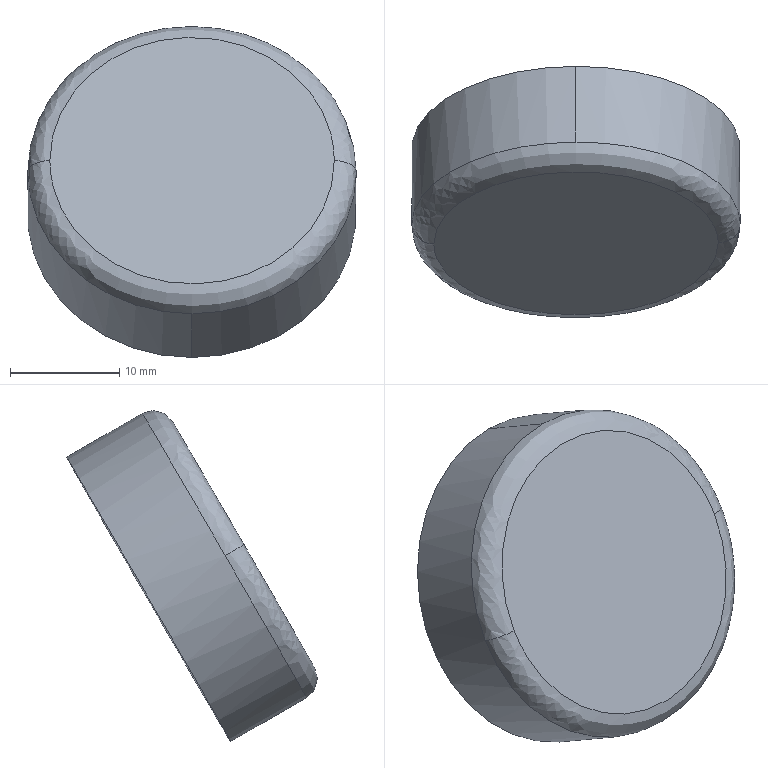Part | SolidWorks | features BaseBody 1 | 1 solid | 6 faces | box 30.03 x 22.929 x 30.249 mm | volume 6990 mm3 | spline 2 | cylinder 2 | plane 2 | commonest cylinder face diameters 30 x2
STEP:
#1=CARTESIAN_POINT('',(730.363,3.802,1.248));
#2=VERTEX_POINT('',#1);
#3=CARTESIAN_POINT('',(756.363,3.915,1.248));
#4=VERTEX_POINT('',#3);
#5=CARTESIAN_POINT('',(730.363,3.802,1.248));
#6=CARTESIAN_POINT('',(730.307,16.802,23.765));
#7=CARTESIAN_POINT('',(756.306,16.915,23.765));
#8=CARTESIAN_POINT('',(756.363,3.915,1.248));
#9=(BOUNDED_CURVE()B_SPLINE_CURVE(3,(#5,#6,#7,#8),.UNSPECIFIED.,.F.,.F.)B_SPLINE_CURVE_WITH_KNOTS((4,4),(0.,1.),.UNSPECIFIED.)CURVE()GEOMETRIC_REPRESENTATION_ITEM()RATIONAL_B_SPLINE_CURVE((1.,0.3333,0.3333,1.))REPRESENTATION_ITEM(''));
#10=EDGE_CURVE('',#2,#4,#9,.T.);
#11=ORIENTED_EDGE('',*,*,#10,.T.);
#12=CARTESIAN_POINT('',(758.356,5.656,0.2485));
#13=VERTEX_POINT('',#12);
#14=CARTESIAN_POINT('',(756.356,5.648,0.2485));
#15=DIRECTION('',(-0.002176,0.5,0.866));
#16=DIRECTION('',(1.,0.004352,-0.000000001));
#17=AXIS2_PLACEMENT_3D('',#14,#15,#16);
#18=CIRCLE('',#17,2.);
#19=EDGE_CURVE('',#4,#13,#18,.T.);
#20=ORIENTED_EDGE('',*,*,#19,.T.);
#21=CARTESIAN_POINT('',(743.356,13.091,13.239));
#22=VERTEX_POINT('',#21);
#23=CARTESIAN_POINT('',(743.356,5.591,0.2485));
#24=DIRECTION('',(-0.003769,0.866,-0.5));
#25=DIRECTION('',(0.,0.5,0.866));
#26=AXIS2_PLACEMENT_3D('',#23,#24,#25);
#27=CIRCLE('',#26,15.);
#28=EDGE_CURVE('',#22,#13,#27,.T.);
#29=ORIENTED_EDGE('',*,*,#28,.F.);
#30=CARTESIAN_POINT('',(728.356,5.526,0.2485));
#31=VERTEX_POINT('',#30);
#32=CARTESIAN_POINT('',(743.356,5.591,0.2485));
#33=DIRECTION('',(-0.003769,0.866,-0.5));
#34=DIRECTION('',(0.,0.5,0.866));
#35=AXIS2_PLACEMENT_3D('',#32,#33,#34);
#36=CIRCLE('',#35,15.);
#37=EDGE_CURVE('',#31,#22,#36,.T.);
#38=ORIENTED_EDGE('',*,*,#37,.F.);
#39=CARTESIAN_POINT('',(730.356,5.534,0.2485));
#40=DIRECTION('',(0.002176,-0.5,-0.866));
#41=DIRECTION('',(-1.,-0.004352,0.000000001));
#42=AXIS2_PLACEMENT_3D('',#39,#40,#41);
#43=CIRCLE('',#42,2.);
#44=EDGE_CURVE('',#2,#31,#43,.T.);
#45=ORIENTED_EDGE('',*,*,#44,.F.);
#46=EDGE_LOOP('',(#11,#20,#29,#38,#45));
#47=FACE_OUTER_BOUND('',#46,.T.);
#48=CARTESIAN_POINT('',(756.363,3.915,1.248));
#49=CARTESIAN_POINT('',(756.306,16.915,23.765));
#50=CARTESIAN_POINT('',(730.307,16.802,23.765));
#51=CARTESIAN_POINT('',(730.363,3.802,1.248));
#52=CARTESIAN_POINT('',(757.535,3.921,1.248));
#53=CARTESIAN_POINT('',(757.473,18.092,25.794));
#54=CARTESIAN_POINT('',(729.13,17.969,25.794));
#55=CARTESIAN_POINT('',(729.192,3.797,1.248));
#56=CARTESIAN_POINT('',(758.36,4.642,0.8343));
#57=CARTESIAN_POINT('',(758.295,19.641,26.815));
#58=CARTESIAN_POINT('',(728.295,19.511,26.815));
#59=CARTESIAN_POINT('',(728.36,4.511,0.8343));
#60=CARTESIAN_POINT('',(758.356,5.656,0.2485));
#61=CARTESIAN_POINT('',(758.29,20.656,26.229));
#62=CARTESIAN_POINT('',(728.291,20.526,26.229));
#63=CARTESIAN_POINT('',(728.356,5.526,0.2485));
#64=(BOUNDED_SURFACE()B_SPLINE_SURFACE(3,3,((#48,#49,#50,#51),(#52,#53,#54,#55),(#56,#57,#58,#59),(#60,#61,#62,#63)),.UNSPECIFIED.,.F.,.F.,.T.)B_SPLINE_SURFACE_WITH_KNOTS((4,4),(4,4),(0.,1.),(0.,1.),.UNSPECIFIED.)GEOMETRIC_REPRESENTATION_ITEM()RATIONAL_B_SPLINE_SURFACE(((1.,0.3333,0.3333,1.),(0.8047,0.2682,0.2682,0.8047),(0.8047,0.2682,0.2682,0.8047),(1.,0.3333,0.3333,1.)))REPRESENTATION_ITEM('')SURFACE());
#65=ADVANCED_FACE('',(#47),#64,.T.);
#66=ORIENTED_EDGE('',*,*,#28,.T.);
#67=CARTESIAN_POINT('',(743.356,-1.909,-12.742));
#68=VERTEX_POINT('',#67);
#69=CARTESIAN_POINT('',(743.356,5.591,0.2485));
#70=DIRECTION('',(-0.003769,0.866,-0.5));
#71=DIRECTION('',(0.,0.5,0.866));
#72=AXIS2_PLACEMENT_3D('',#69,#70,#71);
#73=CIRCLE('',#72,15.);
#74=EDGE_CURVE('',#13,#68,#73,.T.);
#75=ORIENTED_EDGE('',*,*,#74,.T.);
#76=CARTESIAN_POINT('',(743.326,5.019,-16.742));
#77=VERTEX_POINT('',#76);
#78=CARTESIAN_POINT('',(743.326,5.019,-16.742));
#79=DIRECTION('',(-0.003769,0.866,-0.5));
#80=VECTOR('',#79,1000.);
#81=LINE('',#78,#80);
#82=EDGE_CURVE('',#68,#77,#81,.T.);
#83=ORIENTED_EDGE('',*,*,#82,.T.);
#84=CARTESIAN_POINT('',(743.326,20.019,9.239));
#85=VERTEX_POINT('',#84);
#86=CARTESIAN_POINT('',(743.326,12.519,-3.752));
#87=DIRECTION('',(0.003769,-0.866,0.5));
#88=DIRECTION('',(0.,0.5,0.866));
#89=AXIS2_PLACEMENT_3D('',#86,#87,#88);
#90=CIRCLE('',#89,15.);
#91=EDGE_CURVE('',#77,#85,#90,.T.);
#92=ORIENTED_EDGE('',*,*,#91,.T.);
#93=CARTESIAN_POINT('',(743.326,20.019,9.239));
#94=DIRECTION('',(-0.003769,0.866,-0.5));
#95=VECTOR('',#94,1000.);
#96=LINE('',#93,#95);
#97=EDGE_CURVE('',#22,#85,#96,.T.);
#98=ORIENTED_EDGE('',*,*,#97,.F.);
#99=EDGE_LOOP('',(#66,#75,#83,#92,#98));
#100=FACE_OUTER_BOUND('',#99,.T.);
#101=CARTESIAN_POINT('',(743.326,12.519,-3.752));
#102=DIRECTION('',(-0.003769,0.866,-0.5));
#103=DIRECTION('',(0.,0.5,0.866));
#104=AXIS2_PLACEMENT_3D('',#101,#102,#103);
#105=CYLINDRICAL_SURFACE('',#104,15.);
#106=ADVANCED_FACE('',(#100),#105,.T.);
#107=CARTESIAN_POINT('',(743.326,12.519,-3.752));
#108=DIRECTION('',(0.003769,-0.866,0.5));
#109=DIRECTION('',(0.,0.5,0.866));
#110=AXIS2_PLACEMENT_3D('',#107,#108,#109);
#111=CIRCLE('',#110,15.);
#112=EDGE_CURVE('',#85,#77,#111,.T.);
#113=ORIENTED_EDGE('',*,*,#112,.F.);
#114=ORIENTED_EDGE('',*,*,#91,.F.);
#115=EDGE_LOOP('',(#113,#114));
#116=FACE_OUTER_BOUND('',#115,.T.);
#117=CARTESIAN_POINT('',(743.326,12.519,-3.752));
#118=DIRECTION('',(0.003769,-0.866,0.5));
#119=DIRECTION('',(0.,-0.5,-0.866));
#120=AXIS2_PLACEMENT_3D('',#117,#118,#119);
#121=PLANE('',#120);
#122=ADVANCED_FACE('',(#116),#121,.F.);
#123=ORIENTED_EDGE('',*,*,#82,.F.);
#124=CARTESIAN_POINT('',(743.356,5.591,0.2485));
#125=DIRECTION('',(-0.003769,0.866,-0.5));
#126=DIRECTION('',(0.,0.5,0.866));
#127=AXIS2_PLACEMENT_3D('',#124,#125,#126);
#128=CIRCLE('',#127,15.);
#129=EDGE_CURVE('',#68,#31,#128,.T.);
#130=ORIENTED_EDGE('',*,*,#129,.T.);
#131=ORIENTED_EDGE('',*,*,#37,.T.);
#132=ORIENTED_EDGE('',*,*,#97,.T.);
#133=ORIENTED_EDGE('',*,*,#112,.T.);
#134=EDGE_LOOP('',(#123,#130,#131,#132,#133));
#135=FACE_OUTER_BOUND('',#134,.T.);
#136=CARTESIAN_POINT('',(743.326,12.519,-3.752));
#137=DIRECTION('',(-0.003769,0.866,-0.5));
#138=DIRECTION('',(0.,0.5,0.866));
#139=AXIS2_PLACEMENT_3D('',#136,#137,#138);
#140=CYLINDRICAL_SURFACE('',#139,15.);
#141=ADVANCED_FACE('',(#135),#140,.T.);
#142=ORIENTED_EDGE('',*,*,#19,.F.);
#143=CARTESIAN_POINT('',(756.363,3.915,1.248));
#144=CARTESIAN_POINT('',(756.42,-9.084,-21.268));
#145=CARTESIAN_POINT('',(730.42,-9.198,-21.268));
#146=CARTESIAN_POINT('',(730.363,3.802,1.248));
#147=(BOUNDED_CURVE()B_SPLINE_CURVE(3,(#143,#144,#145,#146),.UNSPECIFIED.,.F.,.T.)B_SPLINE_CURVE_WITH_KNOTS((4,4),(0.,1.),.UNSPECIFIED.)CURVE()GEOMETRIC_REPRESENTATION_ITEM()RATIONAL_B_SPLINE_CURVE((1.,0.3333,0.3333,1.))REPRESENTATION_ITEM(''));
#148=EDGE_CURVE('',#4,#2,#147,.T.);
#149=ORIENTED_EDGE('',*,*,#148,.T.);
#150=ORIENTED_EDGE('',*,*,#44,.T.);
#151=ORIENTED_EDGE('',*,*,#129,.F.);
#152=ORIENTED_EDGE('',*,*,#74,.F.);
#153=EDGE_LOOP('',(#142,#149,#150,#151,#152));
#154=FACE_OUTER_BOUND('',#153,.T.);
#155=CARTESIAN_POINT('',(730.363,3.802,1.248));
#156=CARTESIAN_POINT('',(730.42,-9.198,-21.268));
#157=CARTESIAN_POINT('',(756.42,-9.084,-21.268));
#158=CARTESIAN_POINT('',(756.363,3.915,1.248));
#159=CARTESIAN_POINT('',(729.192,3.797,1.248));
#160=CARTESIAN_POINT('',(729.253,-10.374,-23.297));
#161=CARTESIAN_POINT('',(757.596,-10.251,-23.297));
#162=CARTESIAN_POINT('',(757.535,3.921,1.248));
#163=CARTESIAN_POINT('',(728.36,4.511,0.8343));
#164=CARTESIAN_POINT('',(728.425,-10.489,-25.147));
#165=CARTESIAN_POINT('',(758.425,-10.358,-25.147));
#166=CARTESIAN_POINT('',(758.36,4.642,0.8343));
#167=CARTESIAN_POINT('',(728.356,5.526,0.2485));
#168=CARTESIAN_POINT('',(728.421,-9.474,-25.732));
#169=CARTESIAN_POINT('',(758.421,-9.344,-25.732));
#170=CARTESIAN_POINT('',(758.356,5.656,0.2485));
#171=(BOUNDED_SURFACE()B_SPLINE_SURFACE(3,3,((#155,#156,#157,#158),(#159,#160,#161,#162),(#163,#164,#165,#166),(#167,#168,#169,#170)),.UNSPECIFIED.,.F.,.F.,.F.)B_SPLINE_SURFACE_WITH_KNOTS((4,4),(4,4),(0.,1.),(0.,1.),.UNSPECIFIED.)GEOMETRIC_REPRESENTATION_ITEM()RATIONAL_B_SPLINE_SURFACE(((1.,0.3333,0.3333,1.),(0.8047,0.2682,0.2682,0.8047),(0.8047,0.2682,0.2682,0.8047),(1.,0.3333,0.3333,1.)))REPRESENTATION_ITEM('')SURFACE());
#172=ADVANCED_FACE('',(#154),#171,.T.);
#173=ORIENTED_EDGE('',*,*,#148,.F.);
#174=ORIENTED_EDGE('',*,*,#10,.F.);
#175=EDGE_LOOP('',(#173,#174));
#176=FACE_OUTER_BOUND('',#175,.T.);
#177=CARTESIAN_POINT('',(743.363,3.859,1.248));
#178=DIRECTION('',(0.003769,-0.866,0.5));
#179=DIRECTION('',(0.,-0.5,-0.866));
#180=AXIS2_PLACEMENT_3D('',#177,#178,#179);
#181=PLANE('',#180);
#182=ADVANCED_FACE('',(#176),#181,.T.);
#183=CLOSED_SHELL('',(#65,#106,#122,#141,#172,#182));
#184=MANIFOLD_SOLID_BREP('',#183);
#185=CARTESIAN_POINT('',(0.,0.,0.));
#186=DIRECTION('',(0.,0.,1.));
#187=DIRECTION('',(1.,0.,0.));
#188=AXIS2_PLACEMENT_3D('',#185,#186,#187);
#189=(LENGTH_UNIT()NAMED_UNIT(*)SI_UNIT(.MILLI.,.METRE.));
#190=UNCERTAINTY_MEASURE_WITH_UNIT(LENGTH_MEASURE(0.00001),#189,'','');
#191=(NAMED_UNIT(*)PLANE_ANGLE_UNIT()SI_UNIT($,.RADIAN.));
#192=(NAMED_UNIT(*)SI_UNIT($,.STERADIAN.)SOLID_ANGLE_UNIT());
#193=(GEOMETRIC_REPRESENTATION_CONTEXT(3)GLOBAL_UNCERTAINTY_ASSIGNED_CONTEXT((#190))GLOBAL_UNIT_ASSIGNED_CONTEXT((#189,#191,#192))REPRESENTATION_CONTEXT('',''));
#194=ADVANCED_BREP_SHAPE_REPRESENTATION('',(#184,#188),#193);